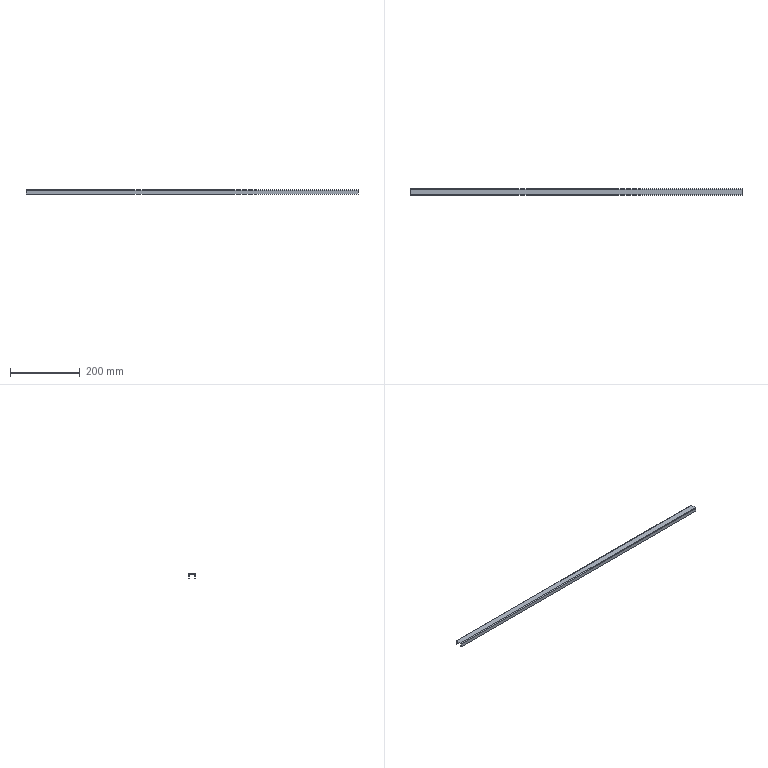Part | SolidWorks | features EdgeFlange 1, FlatPattern 1, SMBaseFlange 1, SheetMetal 1 | 1 solid | 22 faces | box 950 x 20 x 12 mm | volume 74206 mm3 | plane 18 | cylinder 4 | commonest cylinder face diameters 0.2 x2 4.2 x2
STEP:
#1=CARTESIAN_POINT('',(-475.,-7.9,-2.));
#2=VERTEX_POINT('',#1);
#3=CARTESIAN_POINT('',(475.,-7.9,-2.));
#4=VERTEX_POINT('',#3);
#5=CARTESIAN_POINT('',(-475.,-7.9,-2.));
#6=DIRECTION('',(1.,0.,0.));
#7=VECTOR('',#6,1000.);
#8=LINE('',#5,#7);
#9=EDGE_CURVE('',#2,#4,#8,.T.);
#10=ORIENTED_EDGE('',*,*,#9,.F.);
#11=CARTESIAN_POINT('',(-475.,7.9,-2.));
#12=VERTEX_POINT('',#11);
#13=CARTESIAN_POINT('',(-475.,10.,-2.));
#14=DIRECTION('',(0.,-1.,0.));
#15=VECTOR('',#14,1000.);
#16=LINE('',#13,#15);
#17=EDGE_CURVE('',#12,#2,#16,.T.);
#18=ORIENTED_EDGE('',*,*,#17,.F.);
#19=CARTESIAN_POINT('',(475.,7.9,-2.));
#20=VERTEX_POINT('',#19);
#21=CARTESIAN_POINT('',(475.,7.9,-2.));
#22=DIRECTION('',(-1.,0.,0.));
#23=VECTOR('',#22,1000.);
#24=LINE('',#21,#23);
#25=EDGE_CURVE('',#20,#12,#24,.T.);
#26=ORIENTED_EDGE('',*,*,#25,.F.);
#27=CARTESIAN_POINT('',(475.,10.,-2.));
#28=DIRECTION('',(0.,1.,0.));
#29=VECTOR('',#28,1000.);
#30=LINE('',#27,#29);
#31=EDGE_CURVE('',#4,#20,#30,.T.);
#32=ORIENTED_EDGE('',*,*,#31,.F.);
#33=EDGE_LOOP('',(#10,#18,#26,#32));
#34=FACE_OUTER_BOUND('',#33,.T.);
#35=CARTESIAN_POINT('',(0.,0.,-2.));
#36=DIRECTION('',(0.,0.,1.));
#37=DIRECTION('',(1.,0.,0.));
#38=AXIS2_PLACEMENT_3D('',#35,#36,#37);
#39=PLANE('',#38);
#40=ADVANCED_FACE('',(#34),#39,.F.);
#41=CARTESIAN_POINT('',(-475.,7.9,0.));
#42=VERTEX_POINT('',#41);
#43=CARTESIAN_POINT('',(-475.,-7.9,0.));
#44=VERTEX_POINT('',#43);
#45=CARTESIAN_POINT('',(-475.,10.,0.));
#46=DIRECTION('',(0.,-1.,0.));
#47=VECTOR('',#46,1000.);
#48=LINE('',#45,#47);
#49=EDGE_CURVE('',#42,#44,#48,.T.);
#50=ORIENTED_EDGE('',*,*,#49,.T.);
#51=CARTESIAN_POINT('',(475.,-7.9,0.));
#52=VERTEX_POINT('',#51);
#53=CARTESIAN_POINT('',(-475.,-7.9,0.));
#54=DIRECTION('',(1.,0.,0.));
#55=VECTOR('',#54,1000.);
#56=LINE('',#53,#55);
#57=EDGE_CURVE('',#44,#52,#56,.T.);
#58=ORIENTED_EDGE('',*,*,#57,.T.);
#59=CARTESIAN_POINT('',(475.,7.9,0.));
#60=VERTEX_POINT('',#59);
#61=CARTESIAN_POINT('',(475.,10.,0.));
#62=DIRECTION('',(0.,1.,0.));
#63=VECTOR('',#62,1000.);
#64=LINE('',#61,#63);
#65=EDGE_CURVE('',#52,#60,#64,.T.);
#66=ORIENTED_EDGE('',*,*,#65,.T.);
#67=CARTESIAN_POINT('',(475.,7.9,0.));
#68=DIRECTION('',(-1.,0.,0.));
#69=VECTOR('',#68,1000.);
#70=LINE('',#67,#69);
#71=EDGE_CURVE('',#60,#42,#70,.T.);
#72=ORIENTED_EDGE('',*,*,#71,.T.);
#73=EDGE_LOOP('',(#50,#58,#66,#72));
#74=FACE_OUTER_BOUND('',#73,.T.);
#75=CARTESIAN_POINT('',(0.,0.,0.));
#76=DIRECTION('',(0.,0.,1.));
#77=DIRECTION('',(1.,0.,0.));
#78=AXIS2_PLACEMENT_3D('',#75,#76,#77);
#79=PLANE('',#78);
#80=ADVANCED_FACE('',(#74),#79,.T.);
#81=ORIENTED_EDGE('',*,*,#17,.T.);
#82=CARTESIAN_POINT('',(-475.,-7.9,-2.));
#83=DIRECTION('',(0.,0.,1.));
#84=VECTOR('',#83,1000.);
#85=LINE('',#82,#84);
#86=EDGE_CURVE('',#2,#44,#85,.T.);
#87=ORIENTED_EDGE('',*,*,#86,.T.);
#88=ORIENTED_EDGE('',*,*,#49,.F.);
#89=CARTESIAN_POINT('',(-475.,7.9,-2.));
#90=DIRECTION('',(0.,0.,1.));
#91=VECTOR('',#90,1000.);
#92=LINE('',#89,#91);
#93=EDGE_CURVE('',#12,#42,#92,.T.);
#94=ORIENTED_EDGE('',*,*,#93,.F.);
#95=EDGE_LOOP('',(#81,#87,#88,#94));
#96=FACE_OUTER_BOUND('',#95,.T.);
#97=CARTESIAN_POINT('',(-475.,10.,-2.));
#98=DIRECTION('',(-1.,0.,0.));
#99=DIRECTION('',(0.,0.,1.));
#100=AXIS2_PLACEMENT_3D('',#97,#98,#99);
#101=PLANE('',#100);
#102=ADVANCED_FACE('',(#96),#101,.T.);
#103=CARTESIAN_POINT('',(475.,-7.9,-2.));
#104=DIRECTION('',(0.,0.,1.));
#105=VECTOR('',#104,1000.);
#106=LINE('',#103,#105);
#107=EDGE_CURVE('',#4,#52,#106,.T.);
#108=ORIENTED_EDGE('',*,*,#107,.F.);
#109=ORIENTED_EDGE('',*,*,#31,.T.);
#110=CARTESIAN_POINT('',(475.,7.9,-2.));
#111=DIRECTION('',(0.,0.,1.));
#112=VECTOR('',#111,1000.);
#113=LINE('',#110,#112);
#114=EDGE_CURVE('',#20,#60,#113,.T.);
#115=ORIENTED_EDGE('',*,*,#114,.T.);
#116=ORIENTED_EDGE('',*,*,#65,.F.);
#117=EDGE_LOOP('',(#108,#109,#115,#116));
#118=FACE_OUTER_BOUND('',#117,.T.);
#119=CARTESIAN_POINT('',(475.,10.,-2.));
#120=DIRECTION('',(1.,0.,0.));
#121=DIRECTION('',(0.,0.,-1.));
#122=AXIS2_PLACEMENT_3D('',#119,#120,#121);
#123=PLANE('',#122);
#124=ADVANCED_FACE('',(#118),#123,.T.);
#125=CARTESIAN_POINT('',(-475.,8.,-2.1));
#126=VERTEX_POINT('',#125);
#127=CARTESIAN_POINT('',(-475.,10.,-2.1));
#128=VERTEX_POINT('',#127);
#129=CARTESIAN_POINT('',(-475.,10.,-2.1));
#130=DIRECTION('',(0.,1.,0.));
#131=VECTOR('',#130,1000.);
#132=LINE('',#129,#131);
#133=EDGE_CURVE('',#126,#128,#132,.T.);
#134=ORIENTED_EDGE('',*,*,#133,.F.);
#135=CARTESIAN_POINT('',(-475.,7.9,-2.1));
#136=DIRECTION('',(-1.,0.,0.));
#137=DIRECTION('',(0.,0.,-1.));
#138=AXIS2_PLACEMENT_3D('',#135,#136,#137);
#139=CIRCLE('',#138,0.1);
#140=EDGE_CURVE('',#12,#126,#139,.T.);
#141=ORIENTED_EDGE('',*,*,#140,.F.);
#142=ORIENTED_EDGE('',*,*,#93,.T.);
#143=CARTESIAN_POINT('',(-475.,7.9,-2.1));
#144=DIRECTION('',(-1.,0.,0.));
#145=DIRECTION('',(0.,0.,-1.));
#146=AXIS2_PLACEMENT_3D('',#143,#144,#145);
#147=CIRCLE('',#146,2.1);
#148=EDGE_CURVE('',#42,#128,#147,.T.);
#149=ORIENTED_EDGE('',*,*,#148,.T.);
#150=EDGE_LOOP('',(#134,#141,#142,#149));
#151=FACE_OUTER_BOUND('',#150,.T.);
#152=CARTESIAN_POINT('',(-475.,7.9,-2.1));
#153=DIRECTION('',(-1.,0.,0.));
#154=DIRECTION('',(0.,0.,1.));
#155=AXIS2_PLACEMENT_3D('',#152,#153,#154);
#156=PLANE('',#155);
#157=ADVANCED_FACE('',(#151),#156,.T.);
#158=CARTESIAN_POINT('',(475.,8.,-2.1));
#159=VERTEX_POINT('',#158);
#160=CARTESIAN_POINT('',(475.,7.9,-2.1));
#161=DIRECTION('',(1.,0.,0.));
#162=DIRECTION('',(0.,0.,-1.));
#163=AXIS2_PLACEMENT_3D('',#160,#161,#162);
#164=CIRCLE('',#163,0.1);
#165=EDGE_CURVE('',#159,#20,#164,.T.);
#166=ORIENTED_EDGE('',*,*,#165,.F.);
#167=CARTESIAN_POINT('',(475.,10.,-2.1));
#168=VERTEX_POINT('',#167);
#169=CARTESIAN_POINT('',(475.,8.,-2.1));
#170=DIRECTION('',(0.,1.,0.));
#171=VECTOR('',#170,1000.);
#172=LINE('',#169,#171);
#173=EDGE_CURVE('',#159,#168,#172,.T.);
#174=ORIENTED_EDGE('',*,*,#173,.T.);
#175=CARTESIAN_POINT('',(475.,7.9,-2.1));
#176=DIRECTION('',(1.,0.,0.));
#177=DIRECTION('',(0.,0.,-1.));
#178=AXIS2_PLACEMENT_3D('',#175,#176,#177);
#179=CIRCLE('',#178,2.1);
#180=EDGE_CURVE('',#168,#60,#179,.T.);
#181=ORIENTED_EDGE('',*,*,#180,.T.);
#182=ORIENTED_EDGE('',*,*,#114,.F.);
#183=EDGE_LOOP('',(#166,#174,#181,#182));
#184=FACE_OUTER_BOUND('',#183,.T.);
#185=CARTESIAN_POINT('',(475.,7.9,-2.1));
#186=DIRECTION('',(-1.,0.,0.));
#187=DIRECTION('',(0.,0.,1.));
#188=AXIS2_PLACEMENT_3D('',#185,#186,#187);
#189=PLANE('',#188);
#190=ADVANCED_FACE('',(#184),#189,.F.);
#191=ORIENTED_EDGE('',*,*,#71,.F.);
#192=ORIENTED_EDGE('',*,*,#180,.F.);
#193=CARTESIAN_POINT('',(0.,10.,-2.1));
#194=DIRECTION('',(1.,0.,0.));
#195=VECTOR('',#194,1000.);
#196=LINE('',#193,#195);
#197=EDGE_CURVE('',#128,#168,#196,.T.);
#198=ORIENTED_EDGE('',*,*,#197,.F.);
#199=ORIENTED_EDGE('',*,*,#148,.F.);
#200=EDGE_LOOP('',(#191,#192,#198,#199));
#201=FACE_OUTER_BOUND('',#200,.T.);
#202=CARTESIAN_POINT('',(475.,7.9,-2.1));
#203=DIRECTION('',(1.,0.,0.));
#204=DIRECTION('',(0.,1.,0.));
#205=AXIS2_PLACEMENT_3D('',#202,#203,#204);
#206=CYLINDRICAL_SURFACE('',#205,2.1);
#207=ADVANCED_FACE('',(#201),#206,.T.);
#208=ORIENTED_EDGE('',*,*,#25,.T.);
#209=ORIENTED_EDGE('',*,*,#140,.T.);
#210=CARTESIAN_POINT('',(-475.,8.,-2.1));
#211=DIRECTION('',(1.,0.,0.));
#212=VECTOR('',#211,1000.);
#213=LINE('',#210,#212);
#214=EDGE_CURVE('',#126,#159,#213,.T.);
#215=ORIENTED_EDGE('',*,*,#214,.T.);
#216=ORIENTED_EDGE('',*,*,#165,.T.);
#217=EDGE_LOOP('',(#208,#209,#215,#216));
#218=FACE_OUTER_BOUND('',#217,.T.);
#219=CARTESIAN_POINT('',(475.,7.9,-2.1));
#220=DIRECTION('',(1.,0.,0.));
#221=DIRECTION('',(0.,1.,0.));
#222=AXIS2_PLACEMENT_3D('',#219,#220,#221);
#223=CYLINDRICAL_SURFACE('',#222,0.1);
#224=ADVANCED_FACE('',(#218),#223,.F.);
#225=CARTESIAN_POINT('',(475.,10.,-12.));
#226=VERTEX_POINT('',#225);
#227=CARTESIAN_POINT('',(475.,10.,-2.));
#228=DIRECTION('',(0.,0.,1.));
#229=VECTOR('',#228,1000.);
#230=LINE('',#227,#229);
#231=EDGE_CURVE('',#226,#168,#230,.T.);
#232=ORIENTED_EDGE('',*,*,#231,.T.);
#233=ORIENTED_EDGE('',*,*,#173,.F.);
#234=CARTESIAN_POINT('',(475.,8.,-12.));
#235=VERTEX_POINT('',#234);
#236=CARTESIAN_POINT('',(475.,8.,0.));
#237=DIRECTION('',(0.,0.,1.));
#238=VECTOR('',#237,1000.);
#239=LINE('',#236,#238);
#240=EDGE_CURVE('',#235,#159,#239,.T.);
#241=ORIENTED_EDGE('',*,*,#240,.F.);
#242=CARTESIAN_POINT('',(475.,10.,-12.));
#243=DIRECTION('',(0.,-1.,0.));
#244=VECTOR('',#243,1000.);
#245=LINE('',#242,#244);
#246=EDGE_CURVE('',#226,#235,#245,.T.);
#247=ORIENTED_EDGE('',*,*,#246,.F.);
#248=EDGE_LOOP('',(#232,#233,#241,#247));
#249=FACE_OUTER_BOUND('',#248,.T.);
#250=CARTESIAN_POINT('',(475.,10.,-2.));
#251=DIRECTION('',(1.,0.,0.));
#252=DIRECTION('',(0.,0.,-1.));
#253=AXIS2_PLACEMENT_3D('',#250,#251,#252);
#254=PLANE('',#253);
#255=ADVANCED_FACE('',(#249),#254,.T.);
#256=CARTESIAN_POINT('',(-475.,8.,-12.));
#257=VERTEX_POINT('',#256);
#258=CARTESIAN_POINT('',(-475.,8.,0.));
#259=DIRECTION('',(0.,0.,-1.));
#260=VECTOR('',#259,1000.);
#261=LINE('',#258,#260);
#262=EDGE_CURVE('',#126,#257,#261,.T.);
#263=ORIENTED_EDGE('',*,*,#262,.F.);
#264=ORIENTED_EDGE('',*,*,#133,.T.);
#265=CARTESIAN_POINT('',(-475.,10.,-12.));
#266=VERTEX_POINT('',#265);
#267=CARTESIAN_POINT('',(-475.,10.,-12.));
#268=DIRECTION('',(0.,0.,-1.));
#269=VECTOR('',#268,1000.);
#270=LINE('',#267,#269);
#271=EDGE_CURVE('',#128,#266,#270,.T.);
#272=ORIENTED_EDGE('',*,*,#271,.T.);
#273=CARTESIAN_POINT('',(-475.,10.,-12.));
#274=DIRECTION('',(0.,-1.,0.));
#275=VECTOR('',#274,1000.);
#276=LINE('',#273,#275);
#277=EDGE_CURVE('',#266,#257,#276,.T.);
#278=ORIENTED_EDGE('',*,*,#277,.T.);
#279=EDGE_LOOP('',(#263,#264,#272,#278));
#280=FACE_OUTER_BOUND('',#279,.T.);
#281=CARTESIAN_POINT('',(-475.,10.,-12.));
#282=DIRECTION('',(-1.,0.,0.));
#283=DIRECTION('',(0.,0.,1.));
#284=AXIS2_PLACEMENT_3D('',#281,#282,#283);
#285=PLANE('',#284);
#286=ADVANCED_FACE('',(#280),#285,.T.);
#287=ORIENTED_EDGE('',*,*,#271,.F.);
#288=ORIENTED_EDGE('',*,*,#197,.T.);
#289=ORIENTED_EDGE('',*,*,#231,.F.);
#290=CARTESIAN_POINT('',(475.,10.,-12.));
#291=DIRECTION('',(1.,0.,0.));
#292=VECTOR('',#291,1000.);
#293=LINE('',#290,#292);
#294=EDGE_CURVE('',#266,#226,#293,.T.);
#295=ORIENTED_EDGE('',*,*,#294,.F.);
#296=EDGE_LOOP('',(#287,#288,#289,#295));
#297=FACE_OUTER_BOUND('',#296,.T.);
#298=CARTESIAN_POINT('',(0.,10.,0.));
#299=DIRECTION('',(0.,1.,0.));
#300=DIRECTION('',(0.,0.,1.));
#301=AXIS2_PLACEMENT_3D('',#298,#299,#300);
#302=PLANE('',#301);
#303=ADVANCED_FACE('',(#297),#302,.T.);
#304=ORIENTED_EDGE('',*,*,#214,.F.);
#305=ORIENTED_EDGE('',*,*,#262,.T.);
#306=CARTESIAN_POINT('',(0.,8.,-12.));
#307=DIRECTION('',(1.,0.,0.));
#308=VECTOR('',#307,1000.);
#309=LINE('',#306,#308);
#310=EDGE_CURVE('',#257,#235,#309,.T.);
#311=ORIENTED_EDGE('',*,*,#310,.T.);
#312=ORIENTED_EDGE('',*,*,#240,.T.);
#313=EDGE_LOOP('',(#304,#305,#311,#312));
#314=FACE_OUTER_BOUND('',#313,.T.);
#315=CARTESIAN_POINT('',(0.,8.,0.));
#316=DIRECTION('',(0.,1.,0.));
#317=DIRECTION('',(0.,0.,1.));
#318=AXIS2_PLACEMENT_3D('',#315,#316,#317);
#319=PLANE('',#318);
#320=ADVANCED_FACE('',(#314),#319,.F.);
#321=ORIENTED_EDGE('',*,*,#310,.F.);
#322=ORIENTED_EDGE('',*,*,#277,.F.);
#323=ORIENTED_EDGE('',*,*,#294,.T.);
#324=ORIENTED_EDGE('',*,*,#246,.T.);
#325=EDGE_LOOP('',(#321,#322,#323,#324));
#326=FACE_OUTER_BOUND('',#325,.T.);
#327=CARTESIAN_POINT('',(475.,10.,-12.));
#328=DIRECTION('',(0.,0.,-1.));
#329=DIRECTION('',(0.,1.,0.));
#330=AXIS2_PLACEMENT_3D('',#327,#328,#329);
#331=PLANE('',#330);
#332=ADVANCED_FACE('',(#326),#331,.T.);
#333=CARTESIAN_POINT('',(475.,-8.,-2.1));
#334=VERTEX_POINT('',#333);
#335=CARTESIAN_POINT('',(475.,-10.,-2.1));
#336=VERTEX_POINT('',#335);
#337=CARTESIAN_POINT('',(475.,-10.,-2.1));
#338=DIRECTION('',(0.,-1.,0.));
#339=VECTOR('',#338,1000.);
#340=LINE('',#337,#339);
#341=EDGE_CURVE('',#334,#336,#340,.T.);
#342=ORIENTED_EDGE('',*,*,#341,.F.);
#343=CARTESIAN_POINT('',(475.,-7.9,-2.1));
#344=DIRECTION('',(1.,0.,0.));
#345=DIRECTION('',(0.,0.,1.));
#346=AXIS2_PLACEMENT_3D('',#343,#344,#345);
#347=CIRCLE('',#346,0.1);
#348=EDGE_CURVE('',#4,#334,#347,.T.);
#349=ORIENTED_EDGE('',*,*,#348,.F.);
#350=ORIENTED_EDGE('',*,*,#107,.T.);
#351=CARTESIAN_POINT('',(475.,-7.9,-2.1));
#352=DIRECTION('',(1.,0.,0.));
#353=DIRECTION('',(0.,0.,1.));
#354=AXIS2_PLACEMENT_3D('',#351,#352,#353);
#355=CIRCLE('',#354,2.1);
#356=EDGE_CURVE('',#52,#336,#355,.T.);
#357=ORIENTED_EDGE('',*,*,#356,.T.);
#358=EDGE_LOOP('',(#342,#349,#350,#357));
#359=FACE_OUTER_BOUND('',#358,.T.);
#360=CARTESIAN_POINT('',(475.,-7.9,-2.1));
#361=DIRECTION('',(1.,0.,0.));
#362=DIRECTION('',(0.,0.,-1.));
#363=AXIS2_PLACEMENT_3D('',#360,#361,#362);
#364=PLANE('',#363);
#365=ADVANCED_FACE('',(#359),#364,.T.);
#366=CARTESIAN_POINT('',(-475.,-8.,-2.1));
#367=VERTEX_POINT('',#366);
#368=CARTESIAN_POINT('',(-475.,-7.9,-2.1));
#369=DIRECTION('',(-1.,0.,0.));
#370=DIRECTION('',(0.,0.,1.));
#371=AXIS2_PLACEMENT_3D('',#368,#369,#370);
#372=CIRCLE('',#371,0.1);
#373=EDGE_CURVE('',#367,#2,#372,.T.);
#374=ORIENTED_EDGE('',*,*,#373,.F.);
#375=CARTESIAN_POINT('',(-475.,-10.,-2.1));
#376=VERTEX_POINT('',#375);
#377=CARTESIAN_POINT('',(-475.,-8.,-2.1));
#378=DIRECTION('',(0.,-1.,0.));
#379=VECTOR('',#378,1000.);
#380=LINE('',#377,#379);
#381=EDGE_CURVE('',#367,#376,#380,.T.);
#382=ORIENTED_EDGE('',*,*,#381,.T.);
#383=CARTESIAN_POINT('',(-475.,-7.9,-2.1));
#384=DIRECTION('',(-1.,0.,0.));
#385=DIRECTION('',(0.,0.,1.));
#386=AXIS2_PLACEMENT_3D('',#383,#384,#385);
#387=CIRCLE('',#386,2.1);
#388=EDGE_CURVE('',#376,#44,#387,.T.);
#389=ORIENTED_EDGE('',*,*,#388,.T.);
#390=ORIENTED_EDGE('',*,*,#86,.F.);
#391=EDGE_LOOP('',(#374,#382,#389,#390));
#392=FACE_OUTER_BOUND('',#391,.T.);
#393=CARTESIAN_POINT('',(-475.,-7.9,-2.1));
#394=DIRECTION('',(1.,0.,0.));
#395=DIRECTION('',(0.,0.,-1.));
#396=AXIS2_PLACEMENT_3D('',#393,#394,#395);
#397=PLANE('',#396);
#398=ADVANCED_FACE('',(#392),#397,.F.);
#399=ORIENTED_EDGE('',*,*,#57,.F.);
#400=ORIENTED_EDGE('',*,*,#388,.F.);
#401=CARTESIAN_POINT('',(475.,-10.,-2.1));
#402=DIRECTION('',(1.,0.,0.));
#403=VECTOR('',#402,1000.);
#404=LINE('',#401,#403);
#405=EDGE_CURVE('',#376,#336,#404,.T.);
#406=ORIENTED_EDGE('',*,*,#405,.T.);
#407=ORIENTED_EDGE('',*,*,#356,.F.);
#408=EDGE_LOOP('',(#399,#400,#406,#407));
#409=FACE_OUTER_BOUND('',#408,.T.);
#410=CARTESIAN_POINT('',(-475.,-7.9,-2.1));
#411=DIRECTION('',(-1.,0.,0.));
#412=DIRECTION('',(0.,-1.,0.));
#413=AXIS2_PLACEMENT_3D('',#410,#411,#412);
#414=CYLINDRICAL_SURFACE('',#413,2.1);
#415=ADVANCED_FACE('',(#409),#414,.T.);
#416=ORIENTED_EDGE('',*,*,#9,.T.);
#417=ORIENTED_EDGE('',*,*,#348,.T.);
#418=CARTESIAN_POINT('',(475.,-8.,-2.1));
#419=DIRECTION('',(-1.,0.,0.));
#420=VECTOR('',#419,1000.);
#421=LINE('',#418,#420);
#422=EDGE_CURVE('',#334,#367,#421,.T.);
#423=ORIENTED_EDGE('',*,*,#422,.T.);
#424=ORIENTED_EDGE('',*,*,#373,.T.);
#425=EDGE_LOOP('',(#416,#417,#423,#424));
#426=FACE_OUTER_BOUND('',#425,.T.);
#427=CARTESIAN_POINT('',(-475.,-7.9,-2.1));
#428=DIRECTION('',(-1.,0.,0.));
#429=DIRECTION('',(0.,-1.,0.));
#430=AXIS2_PLACEMENT_3D('',#427,#428,#429);
#431=CYLINDRICAL_SURFACE('',#430,0.1);
#432=ADVANCED_FACE('',(#426),#431,.F.);
#433=CARTESIAN_POINT('',(475.,-8.,-12.));
#434=VERTEX_POINT('',#433);
#435=CARTESIAN_POINT('',(475.,-8.,0.));
#436=DIRECTION('',(0.,0.,-1.));
#437=VECTOR('',#436,1000.);
#438=LINE('',#435,#437);
#439=EDGE_CURVE('',#334,#434,#438,.T.);
#440=ORIENTED_EDGE('',*,*,#439,.F.);
#441=ORIENTED_EDGE('',*,*,#341,.T.);
#442=CARTESIAN_POINT('',(475.,-10.,-12.));
#443=VERTEX_POINT('',#442);
#444=CARTESIAN_POINT('',(475.,-10.,-2.));
#445=DIRECTION('',(0.,0.,-1.));
#446=VECTOR('',#445,1000.);
#447=LINE('',#444,#446);
#448=EDGE_CURVE('',#336,#443,#447,.T.);
#449=ORIENTED_EDGE('',*,*,#448,.T.);
#450=CARTESIAN_POINT('',(475.,-10.,-12.));
#451=DIRECTION('',(0.,1.,0.));
#452=VECTOR('',#451,1000.);
#453=LINE('',#450,#452);
#454=EDGE_CURVE('',#443,#434,#453,.T.);
#455=ORIENTED_EDGE('',*,*,#454,.T.);
#456=EDGE_LOOP('',(#440,#441,#449,#455));
#457=FACE_OUTER_BOUND('',#456,.T.);
#458=CARTESIAN_POINT('',(475.,-10.,-2.));
#459=DIRECTION('',(1.,0.,0.));
#460=DIRECTION('',(0.,0.,-1.));
#461=AXIS2_PLACEMENT_3D('',#458,#459,#460);
#462=PLANE('',#461);
#463=ADVANCED_FACE('',(#457),#462,.T.);
#464=CARTESIAN_POINT('',(-475.,-10.,-12.));
#465=VERTEX_POINT('',#464);
#466=CARTESIAN_POINT('',(-475.,-10.,-12.));
#467=DIRECTION('',(0.,0.,1.));
#468=VECTOR('',#467,1000.);
#469=LINE('',#466,#468);
#470=EDGE_CURVE('',#465,#376,#469,.T.);
#471=ORIENTED_EDGE('',*,*,#470,.T.);
#472=ORIENTED_EDGE('',*,*,#381,.F.);
#473=CARTESIAN_POINT('',(-475.,-8.,-12.));
#474=VERTEX_POINT('',#473);
#475=CARTESIAN_POINT('',(-475.,-8.,0.));
#476=DIRECTION('',(0.,0.,1.));
#477=VECTOR('',#476,1000.);
#478=LINE('',#475,#477);
#479=EDGE_CURVE('',#474,#367,#478,.T.);
#480=ORIENTED_EDGE('',*,*,#479,.F.);
#481=CARTESIAN_POINT('',(-475.,-10.,-12.));
#482=DIRECTION('',(0.,1.,0.));
#483=VECTOR('',#482,1000.);
#484=LINE('',#481,#483);
#485=EDGE_CURVE('',#465,#474,#484,.T.);
#486=ORIENTED_EDGE('',*,*,#485,.F.);
#487=EDGE_LOOP('',(#471,#472,#480,#486));
#488=FACE_OUTER_BOUND('',#487,.T.);
#489=CARTESIAN_POINT('',(-475.,-10.,-12.));
#490=DIRECTION('',(-1.,0.,0.));
#491=DIRECTION('',(0.,0.,1.));
#492=AXIS2_PLACEMENT_3D('',#489,#490,#491);
#493=PLANE('',#492);
#494=ADVANCED_FACE('',(#488),#493,.T.);
#495=ORIENTED_EDGE('',*,*,#405,.F.);
#496=ORIENTED_EDGE('',*,*,#470,.F.);
#497=CARTESIAN_POINT('',(475.,-10.,-12.));
#498=DIRECTION('',(-1.,0.,0.));
#499=VECTOR('',#498,1000.);
#500=LINE('',#497,#499);
#501=EDGE_CURVE('',#443,#465,#500,.T.);
#502=ORIENTED_EDGE('',*,*,#501,.F.);
#503=ORIENTED_EDGE('',*,*,#448,.F.);
#504=EDGE_LOOP('',(#495,#496,#502,#503));
#505=FACE_OUTER_BOUND('',#504,.T.);
#506=CARTESIAN_POINT('',(0.,-10.,0.));
#507=DIRECTION('',(0.,1.,0.));
#508=DIRECTION('',(0.,0.,1.));
#509=AXIS2_PLACEMENT_3D('',#506,#507,#508);
#510=PLANE('',#509);
#511=ADVANCED_FACE('',(#505),#510,.F.);
#512=ORIENTED_EDGE('',*,*,#479,.T.);
#513=ORIENTED_EDGE('',*,*,#422,.F.);
#514=ORIENTED_EDGE('',*,*,#439,.T.);
#515=CARTESIAN_POINT('',(0.,-8.,-12.));
#516=DIRECTION('',(-1.,0.,0.));
#517=VECTOR('',#516,1000.);
#518=LINE('',#515,#517);
#519=EDGE_CURVE('',#434,#474,#518,.T.);
#520=ORIENTED_EDGE('',*,*,#519,.T.);
#521=EDGE_LOOP('',(#512,#513,#514,#520));
#522=FACE_OUTER_BOUND('',#521,.T.);
#523=CARTESIAN_POINT('',(0.,-8.,0.));
#524=DIRECTION('',(0.,1.,0.));
#525=DIRECTION('',(0.,0.,1.));
#526=AXIS2_PLACEMENT_3D('',#523,#524,#525);
#527=PLANE('',#526);
#528=ADVANCED_FACE('',(#522),#527,.T.);
#529=ORIENTED_EDGE('',*,*,#519,.F.);
#530=ORIENTED_EDGE('',*,*,#454,.F.);
#531=ORIENTED_EDGE('',*,*,#501,.T.);
#532=ORIENTED_EDGE('',*,*,#485,.T.);
#533=EDGE_LOOP('',(#529,#530,#531,#532));
#534=FACE_OUTER_BOUND('',#533,.T.);
#535=CARTESIAN_POINT('',(475.,-10.,-12.));
#536=DIRECTION('',(0.,0.,-1.));
#537=DIRECTION('',(0.,1.,0.));
#538=AXIS2_PLACEMENT_3D('',#535,#536,#537);
#539=PLANE('',#538);
#540=ADVANCED_FACE('',(#534),#539,.T.);
#541=CLOSED_SHELL('',(#40,#80,#102,#124,#157,#190,#207,#224,#255,#286,#303,#320,#332,#365,#398,#415,#432,#463,#494,#511,#528,#540));
#542=MANIFOLD_SOLID_BREP('',#541);
#543=CARTESIAN_POINT('',(0.,0.,0.));
#544=DIRECTION('',(0.,0.,1.));
#545=DIRECTION('',(1.,0.,0.));
#546=AXIS2_PLACEMENT_3D('',#543,#544,#545);
#547=(LENGTH_UNIT()NAMED_UNIT(*)SI_UNIT(.MILLI.,.METRE.));
#548=UNCERTAINTY_MEASURE_WITH_UNIT(LENGTH_MEASURE(0.00001),#547,'','');
#549=(NAMED_UNIT(*)PLANE_ANGLE_UNIT()SI_UNIT($,.RADIAN.));
#550=(NAMED_UNIT(*)SI_UNIT($,.STERADIAN.)SOLID_ANGLE_UNIT());
#551=(GEOMETRIC_REPRESENTATION_CONTEXT(3)GLOBAL_UNCERTAINTY_ASSIGNED_CONTEXT((#548))GLOBAL_UNIT_ASSIGNED_CONTEXT((#547,#549,#550))REPRESENTATION_CONTEXT('',''));
#552=ADVANCED_BREP_SHAPE_REPRESENTATION('',(#542,#546),#551);